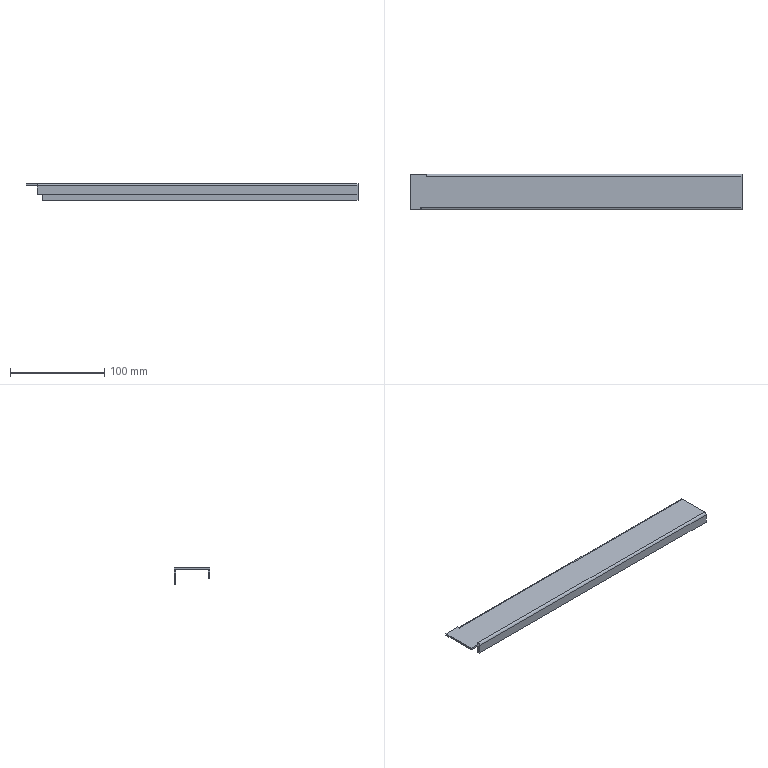Part | STEP file | Electrical Cabinet 5 | 1 solid | 22 faces | box 352 x 38 x 18 mm | volume 43368 mm3 | plane 18 | cylinder 4 | commonest cylinder face diameters 1 x2 5 x2
STEP:
#1=CARTESIAN_POINT('',(-50.375,-23.063,-2.));
#2=VERTEX_POINT('',#1);
#3=CARTESIAN_POINT('',(-38.775,-23.063,-2.));
#4=VERTEX_POINT('',#3);
#5=CARTESIAN_POINT('',(0.,-23.063,-2.));
#6=DIRECTION('',(1.,0.,0.));
#7=VECTOR('',#6,1000.);
#8=LINE('',#5,#7);
#9=EDGE_CURVE('',#2,#4,#8,.T.);
#10=ORIENTED_EDGE('',*,*,#9,.F.);
#11=CARTESIAN_POINT('',(-50.375,14.937,-2.));
#12=VERTEX_POINT('',#11);
#13=CARTESIAN_POINT('',(-50.375,0.,-2.));
#14=DIRECTION('',(0.,-1.,0.));
#15=VECTOR('',#14,1000.);
#16=LINE('',#13,#15);
#17=EDGE_CURVE('',#12,#2,#16,.T.);
#18=ORIENTED_EDGE('',*,*,#17,.F.);
#19=CARTESIAN_POINT('',(-32.775,14.937,-2.));
#20=VERTEX_POINT('',#19);
#21=CARTESIAN_POINT('',(0.,14.937,-2.));
#22=DIRECTION('',(-1.,0.,0.));
#23=VECTOR('',#22,1000.);
#24=LINE('',#21,#23);
#25=EDGE_CURVE('',#20,#12,#24,.T.);
#26=ORIENTED_EDGE('',*,*,#25,.F.);
#27=CARTESIAN_POINT('',(-32.775,12.037,-2.));
#28=VERTEX_POINT('',#27);
#29=CARTESIAN_POINT('',(-32.775,0.,-2.));
#30=DIRECTION('',(0.,1.,0.));
#31=VECTOR('',#30,1000.);
#32=LINE('',#29,#31);
#33=EDGE_CURVE('',#28,#20,#32,.T.);
#34=ORIENTED_EDGE('',*,*,#33,.F.);
#35=CARTESIAN_POINT('',(-32.375,12.037,-2.));
#36=VERTEX_POINT('',#35);
#37=CARTESIAN_POINT('',(-32.375,12.037,-2.));
#38=DIRECTION('',(-1.,0.,0.));
#39=VECTOR('',#38,1000.);
#40=LINE('',#37,#39);
#41=EDGE_CURVE('',#36,#28,#40,.T.);
#42=ORIENTED_EDGE('',*,*,#41,.F.);
#43=CARTESIAN_POINT('',(-32.375,12.437,-2.));
#44=VERTEX_POINT('',#43);
#45=CARTESIAN_POINT('',(-32.375,12.437,-2.));
#46=DIRECTION('',(0.,-1.,0.));
#47=VECTOR('',#46,1000.);
#48=LINE('',#45,#47);
#49=EDGE_CURVE('',#44,#36,#48,.T.);
#50=ORIENTED_EDGE('',*,*,#49,.F.);
#51=CARTESIAN_POINT('',(301.625,12.437,-2.));
#52=VERTEX_POINT('',#51);
#53=CARTESIAN_POINT('',(0.,12.437,-2.));
#54=DIRECTION('',(-1.,0.,0.));
#55=VECTOR('',#54,1000.);
#56=LINE('',#53,#55);
#57=EDGE_CURVE('',#52,#44,#56,.T.);
#58=ORIENTED_EDGE('',*,*,#57,.F.);
#59=CARTESIAN_POINT('',(301.625,-20.563,-2.));
#60=VERTEX_POINT('',#59);
#61=CARTESIAN_POINT('',(301.625,0.,-2.));
#62=DIRECTION('',(0.,1.,0.));
#63=VECTOR('',#62,1000.);
#64=LINE('',#61,#63);
#65=EDGE_CURVE('',#60,#52,#64,.T.);
#66=ORIENTED_EDGE('',*,*,#65,.F.);
#67=CARTESIAN_POINT('',(-38.375,-20.563,-2.));
#68=VERTEX_POINT('',#67);
#69=CARTESIAN_POINT('',(0.,-20.563,-2.));
#70=DIRECTION('',(1.,0.,0.));
#71=VECTOR('',#70,1000.);
#72=LINE('',#69,#71);
#73=EDGE_CURVE('',#68,#60,#72,.T.);
#74=ORIENTED_EDGE('',*,*,#73,.F.);
#75=CARTESIAN_POINT('',(-38.375,-20.163,-2.));
#76=VERTEX_POINT('',#75);
#77=CARTESIAN_POINT('',(-38.375,-20.163,-2.));
#78=DIRECTION('',(0.,-1.,0.));
#79=VECTOR('',#78,1000.);
#80=LINE('',#77,#79);
#81=EDGE_CURVE('',#76,#68,#80,.T.);
#82=ORIENTED_EDGE('',*,*,#81,.F.);
#83=CARTESIAN_POINT('',(-38.775,-20.163,-2.));
#84=VERTEX_POINT('',#83);
#85=CARTESIAN_POINT('',(-38.775,-20.163,-2.));
#86=DIRECTION('',(1.,0.,0.));
#87=VECTOR('',#86,1000.);
#88=LINE('',#85,#87);
#89=EDGE_CURVE('',#84,#76,#88,.T.);
#90=ORIENTED_EDGE('',*,*,#89,.F.);
#91=CARTESIAN_POINT('',(-38.775,0.,-2.));
#92=DIRECTION('',(0.,1.,0.));
#93=VECTOR('',#92,1000.);
#94=LINE('',#91,#93);
#95=EDGE_CURVE('',#4,#84,#94,.T.);
#96=ORIENTED_EDGE('',*,*,#95,.F.);
#97=EDGE_LOOP('',(#10,#18,#26,#34,#42,#50,#58,#66,#74,#82,#90,#96));
#98=FACE_OUTER_BOUND('',#97,.T.);
#99=CARTESIAN_POINT('',(0.,0.,-2.));
#100=DIRECTION('',(0.,0.,1.));
#101=DIRECTION('',(1.,0.,0.));
#102=AXIS2_PLACEMENT_3D('',#99,#100,#101);
#103=PLANE('',#102);
#104=ADVANCED_FACE('',(#98),#103,.F.);
#105=ORIENTED_EDGE('',*,*,#95,.T.);
#106=CARTESIAN_POINT('',(-38.775,-20.163,0.));
#107=VERTEX_POINT('',#106);
#108=CARTESIAN_POINT('',(-38.775,-20.163,-2.));
#109=DIRECTION('',(0.,0.,1.));
#110=VECTOR('',#109,1000.);
#111=LINE('',#108,#110);
#112=EDGE_CURVE('',#84,#107,#111,.T.);
#113=ORIENTED_EDGE('',*,*,#112,.T.);
#114=CARTESIAN_POINT('',(-38.775,-23.063,0.));
#115=VERTEX_POINT('',#114);
#116=CARTESIAN_POINT('',(-38.775,-23.063,0.));
#117=DIRECTION('',(0.,-1.,0.));
#118=VECTOR('',#117,1000.);
#119=LINE('',#116,#118);
#120=EDGE_CURVE('',#107,#115,#119,.T.);
#121=ORIENTED_EDGE('',*,*,#120,.T.);
#122=CARTESIAN_POINT('',(-38.775,-23.063,-2.));
#123=DIRECTION('',(0.,0.,-1.));
#124=VECTOR('',#123,1000.);
#125=LINE('',#122,#124);
#126=EDGE_CURVE('',#115,#4,#125,.T.);
#127=ORIENTED_EDGE('',*,*,#126,.T.);
#128=EDGE_LOOP('',(#105,#113,#121,#127));
#129=FACE_OUTER_BOUND('',#128,.T.);
#130=CARTESIAN_POINT('',(-38.775,-23.063,-2.));
#131=DIRECTION('',(1.,0.,0.));
#132=DIRECTION('',(0.,0.,-1.));
#133=AXIS2_PLACEMENT_3D('',#130,#131,#132);
#134=PLANE('',#133);
#135=ADVANCED_FACE('',(#129),#134,.T.);
#136=CARTESIAN_POINT('',(-50.375,-23.063,0.));
#137=VERTEX_POINT('',#136);
#138=CARTESIAN_POINT('',(-50.375,-23.063,0.));
#139=DIRECTION('',(-1.,0.,0.));
#140=VECTOR('',#139,1000.);
#141=LINE('',#138,#140);
#142=EDGE_CURVE('',#115,#137,#141,.T.);
#143=ORIENTED_EDGE('',*,*,#142,.T.);
#144=CARTESIAN_POINT('',(-50.375,-23.063,-2.));
#145=DIRECTION('',(0.,0.,-1.));
#146=VECTOR('',#145,1000.);
#147=LINE('',#144,#146);
#148=EDGE_CURVE('',#137,#2,#147,.T.);
#149=ORIENTED_EDGE('',*,*,#148,.T.);
#150=ORIENTED_EDGE('',*,*,#9,.T.);
#151=ORIENTED_EDGE('',*,*,#126,.F.);
#152=EDGE_LOOP('',(#143,#149,#150,#151));
#153=FACE_OUTER_BOUND('',#152,.T.);
#154=CARTESIAN_POINT('',(-50.375,-23.063,-2.));
#155=DIRECTION('',(0.,-1.,0.));
#156=DIRECTION('',(0.,0.,-1.));
#157=AXIS2_PLACEMENT_3D('',#154,#155,#156);
#158=PLANE('',#157);
#159=ADVANCED_FACE('',(#153),#158,.T.);
#160=ORIENTED_EDGE('',*,*,#17,.T.);
#161=ORIENTED_EDGE('',*,*,#148,.F.);
#162=CARTESIAN_POINT('',(-50.375,14.937,0.));
#163=VERTEX_POINT('',#162);
#164=CARTESIAN_POINT('',(-50.375,14.937,0.));
#165=DIRECTION('',(0.,1.,0.));
#166=VECTOR('',#165,1000.);
#167=LINE('',#164,#166);
#168=EDGE_CURVE('',#137,#163,#167,.T.);
#169=ORIENTED_EDGE('',*,*,#168,.T.);
#170=CARTESIAN_POINT('',(-50.375,14.937,-2.));
#171=DIRECTION('',(0.,0.,-1.));
#172=VECTOR('',#171,1000.);
#173=LINE('',#170,#172);
#174=EDGE_CURVE('',#163,#12,#173,.T.);
#175=ORIENTED_EDGE('',*,*,#174,.T.);
#176=EDGE_LOOP('',(#160,#161,#169,#175));
#177=FACE_OUTER_BOUND('',#176,.T.);
#178=CARTESIAN_POINT('',(-50.375,14.937,-2.));
#179=DIRECTION('',(-1.,0.,0.));
#180=DIRECTION('',(0.,-1.,0.));
#181=AXIS2_PLACEMENT_3D('',#178,#179,#180);
#182=PLANE('',#181);
#183=ADVANCED_FACE('',(#177),#182,.T.);
#184=ORIENTED_EDGE('',*,*,#25,.T.);
#185=ORIENTED_EDGE('',*,*,#174,.F.);
#186=CARTESIAN_POINT('',(-32.775,14.937,0.));
#187=VERTEX_POINT('',#186);
#188=CARTESIAN_POINT('',(-50.375,14.937,0.));
#189=DIRECTION('',(1.,0.,0.));
#190=VECTOR('',#189,1000.);
#191=LINE('',#188,#190);
#192=EDGE_CURVE('',#163,#187,#191,.T.);
#193=ORIENTED_EDGE('',*,*,#192,.T.);
#194=CARTESIAN_POINT('',(-32.775,14.937,-2.));
#195=DIRECTION('',(0.,0.,-1.));
#196=VECTOR('',#195,1000.);
#197=LINE('',#194,#196);
#198=EDGE_CURVE('',#187,#20,#197,.T.);
#199=ORIENTED_EDGE('',*,*,#198,.T.);
#200=EDGE_LOOP('',(#184,#185,#193,#199));
#201=FACE_OUTER_BOUND('',#200,.T.);
#202=CARTESIAN_POINT('',(-50.375,14.937,-2.));
#203=DIRECTION('',(0.,1.,0.));
#204=DIRECTION('',(0.,0.,1.));
#205=AXIS2_PLACEMENT_3D('',#202,#203,#204);
#206=PLANE('',#205);
#207=ADVANCED_FACE('',(#201),#206,.T.);
#208=ORIENTED_EDGE('',*,*,#33,.T.);
#209=ORIENTED_EDGE('',*,*,#198,.F.);
#210=CARTESIAN_POINT('',(-32.775,12.037,0.));
#211=VERTEX_POINT('',#210);
#212=CARTESIAN_POINT('',(-32.775,12.037,0.));
#213=DIRECTION('',(0.,-1.,0.));
#214=VECTOR('',#213,1000.);
#215=LINE('',#212,#214);
#216=EDGE_CURVE('',#187,#211,#215,.T.);
#217=ORIENTED_EDGE('',*,*,#216,.T.);
#218=CARTESIAN_POINT('',(-32.775,12.037,-2.));
#219=DIRECTION('',(0.,0.,-1.));
#220=VECTOR('',#219,1000.);
#221=LINE('',#218,#220);
#222=EDGE_CURVE('',#211,#28,#221,.T.);
#223=ORIENTED_EDGE('',*,*,#222,.T.);
#224=EDGE_LOOP('',(#208,#209,#217,#223));
#225=FACE_OUTER_BOUND('',#224,.T.);
#226=CARTESIAN_POINT('',(-32.775,12.037,-2.));
#227=DIRECTION('',(1.,0.,0.));
#228=DIRECTION('',(0.,0.,-1.));
#229=AXIS2_PLACEMENT_3D('',#226,#227,#228);
#230=PLANE('',#229);
#231=ADVANCED_FACE('',(#225),#230,.T.);
#232=CARTESIAN_POINT('',(-32.375,12.937,-2.5));
#233=VERTEX_POINT('',#232);
#234=CARTESIAN_POINT('',(-32.375,12.437,-2.5));
#235=DIRECTION('',(1.,0.,0.));
#236=DIRECTION('',(0.,0.,-1.));
#237=AXIS2_PLACEMENT_3D('',#234,#235,#236);
#238=CIRCLE('',#237,0.5);
#239=EDGE_CURVE('',#233,#44,#238,.T.);
#240=ORIENTED_EDGE('',*,*,#239,.F.);
#241=CARTESIAN_POINT('',(301.625,12.937,-2.5));
#242=VERTEX_POINT('',#241);
#243=CARTESIAN_POINT('',(301.625,12.937,-2.5));
#244=DIRECTION('',(-1.,0.,0.));
#245=VECTOR('',#244,1000.);
#246=LINE('',#243,#245);
#247=EDGE_CURVE('',#242,#233,#246,.T.);
#248=ORIENTED_EDGE('',*,*,#247,.F.);
#249=CARTESIAN_POINT('',(301.625,12.437,-2.5));
#250=DIRECTION('',(1.,0.,0.));
#251=DIRECTION('',(0.,0.,-1.));
#252=AXIS2_PLACEMENT_3D('',#249,#250,#251);
#253=CIRCLE('',#252,0.5);
#254=EDGE_CURVE('',#242,#52,#253,.T.);
#255=ORIENTED_EDGE('',*,*,#254,.T.);
#256=ORIENTED_EDGE('',*,*,#57,.T.);
#257=EDGE_LOOP('',(#240,#248,#255,#256));
#258=FACE_OUTER_BOUND('',#257,.T.);
#259=CARTESIAN_POINT('',(301.625,12.437,-2.5));
#260=DIRECTION('',(1.,0.,0.));
#261=DIRECTION('',(0.,0.,-1.));
#262=AXIS2_PLACEMENT_3D('',#259,#260,#261);
#263=CYLINDRICAL_SURFACE('',#262,0.5);
#264=ADVANCED_FACE('',(#258),#263,.F.);
#265=ORIENTED_EDGE('',*,*,#65,.T.);
#266=ORIENTED_EDGE('',*,*,#254,.F.);
#267=CARTESIAN_POINT('',(301.625,12.937,-18.));
#268=VERTEX_POINT('',#267);
#269=CARTESIAN_POINT('',(301.625,12.937,0.));
#270=DIRECTION('',(0.,0.,-1.));
#271=VECTOR('',#270,1000.);
#272=LINE('',#269,#271);
#273=EDGE_CURVE('',#242,#268,#272,.T.);
#274=ORIENTED_EDGE('',*,*,#273,.T.);
#275=CARTESIAN_POINT('',(301.625,14.937,-18.));
#276=VERTEX_POINT('',#275);
#277=CARTESIAN_POINT('',(301.625,14.937,-18.));
#278=DIRECTION('',(0.,-1.,0.));
#279=VECTOR('',#278,1000.);
#280=LINE('',#277,#279);
#281=EDGE_CURVE('',#276,#268,#280,.T.);
#282=ORIENTED_EDGE('',*,*,#281,.F.);
#283=CARTESIAN_POINT('',(301.625,14.937,-2.5));
#284=VERTEX_POINT('',#283);
#285=CARTESIAN_POINT('',(301.625,14.937,-2.));
#286=DIRECTION('',(0.,0.,1.));
#287=VECTOR('',#286,1000.);
#288=LINE('',#285,#287);
#289=EDGE_CURVE('',#276,#284,#288,.T.);
#290=ORIENTED_EDGE('',*,*,#289,.T.);
#291=CARTESIAN_POINT('',(301.625,12.437,0.));
#292=VERTEX_POINT('',#291);
#293=CARTESIAN_POINT('',(301.625,12.437,-2.5));
#294=DIRECTION('',(-1.,0.,0.));
#295=DIRECTION('',(0.,0.,-1.));
#296=AXIS2_PLACEMENT_3D('',#293,#294,#295);
#297=CIRCLE('',#296,2.5);
#298=EDGE_CURVE('',#292,#284,#297,.T.);
#299=ORIENTED_EDGE('',*,*,#298,.F.);
#300=CARTESIAN_POINT('',(301.625,-20.563,0.));
#301=VERTEX_POINT('',#300);
#302=CARTESIAN_POINT('',(301.625,14.937,0.));
#303=DIRECTION('',(0.,-1.,0.));
#304=VECTOR('',#303,1000.);
#305=LINE('',#302,#304);
#306=EDGE_CURVE('',#292,#301,#305,.T.);
#307=ORIENTED_EDGE('',*,*,#306,.T.);
#308=CARTESIAN_POINT('',(301.625,-23.063,-2.5));
#309=VERTEX_POINT('',#308);
#310=CARTESIAN_POINT('',(301.625,-20.563,-2.5));
#311=DIRECTION('',(1.,0.,0.));
#312=DIRECTION('',(0.,0.,1.));
#313=AXIS2_PLACEMENT_3D('',#310,#311,#312);
#314=CIRCLE('',#313,2.5);
#315=EDGE_CURVE('',#301,#309,#314,.T.);
#316=ORIENTED_EDGE('',*,*,#315,.T.);
#317=CARTESIAN_POINT('',(301.625,-23.063,-12.));
#318=VERTEX_POINT('',#317);
#319=CARTESIAN_POINT('',(301.625,-23.063,-2.));
#320=DIRECTION('',(0.,0.,1.));
#321=VECTOR('',#320,1000.);
#322=LINE('',#319,#321);
#323=EDGE_CURVE('',#318,#309,#322,.T.);
#324=ORIENTED_EDGE('',*,*,#323,.F.);
#325=CARTESIAN_POINT('',(301.625,-21.063,-12.));
#326=VERTEX_POINT('',#325);
#327=CARTESIAN_POINT('',(301.625,-23.063,-12.));
#328=DIRECTION('',(0.,-1.,0.));
#329=VECTOR('',#328,1000.);
#330=LINE('',#327,#329);
#331=EDGE_CURVE('',#326,#318,#330,.T.);
#332=ORIENTED_EDGE('',*,*,#331,.F.);
#333=CARTESIAN_POINT('',(301.625,-21.063,-2.5));
#334=VERTEX_POINT('',#333);
#335=CARTESIAN_POINT('',(301.625,-21.063,0.));
#336=DIRECTION('',(0.,0.,-1.));
#337=VECTOR('',#336,1000.);
#338=LINE('',#335,#337);
#339=EDGE_CURVE('',#334,#326,#338,.T.);
#340=ORIENTED_EDGE('',*,*,#339,.F.);
#341=CARTESIAN_POINT('',(301.625,-20.563,-2.5));
#342=DIRECTION('',(-1.,0.,0.));
#343=DIRECTION('',(0.,0.,1.));
#344=AXIS2_PLACEMENT_3D('',#341,#342,#343);
#345=CIRCLE('',#344,0.5);
#346=EDGE_CURVE('',#334,#60,#345,.T.);
#347=ORIENTED_EDGE('',*,*,#346,.T.);
#348=EDGE_LOOP('',(#265,#266,#274,#282,#290,#299,#307,#316,#324,#332,#340,#347));
#349=FACE_OUTER_BOUND('',#348,.T.);
#350=CARTESIAN_POINT('',(301.625,14.937,-2.));
#351=DIRECTION('',(1.,0.,0.));
#352=DIRECTION('',(0.,0.,-1.));
#353=AXIS2_PLACEMENT_3D('',#350,#351,#352);
#354=PLANE('',#353);
#355=ADVANCED_FACE('',(#349),#354,.T.);
#356=ORIENTED_EDGE('',*,*,#346,.F.);
#357=CARTESIAN_POINT('',(-38.375,-21.063,-2.5));
#358=VERTEX_POINT('',#357);
#359=CARTESIAN_POINT('',(-38.375,-21.063,-2.5));
#360=DIRECTION('',(1.,0.,0.));
#361=VECTOR('',#360,1000.);
#362=LINE('',#359,#361);
#363=EDGE_CURVE('',#358,#334,#362,.T.);
#364=ORIENTED_EDGE('',*,*,#363,.F.);
#365=CARTESIAN_POINT('',(-38.375,-20.563,-2.5));
#366=DIRECTION('',(-1.,0.,0.));
#367=DIRECTION('',(0.,0.,1.));
#368=AXIS2_PLACEMENT_3D('',#365,#366,#367);
#369=CIRCLE('',#368,0.5);
#370=EDGE_CURVE('',#358,#68,#369,.T.);
#371=ORIENTED_EDGE('',*,*,#370,.T.);
#372=ORIENTED_EDGE('',*,*,#73,.T.);
#373=EDGE_LOOP('',(#356,#364,#371,#372));
#374=FACE_OUTER_BOUND('',#373,.T.);
#375=CARTESIAN_POINT('',(-38.375,-20.563,-2.5));
#376=DIRECTION('',(-1.,0.,0.));
#377=DIRECTION('',(0.,0.,1.));
#378=AXIS2_PLACEMENT_3D('',#375,#376,#377);
#379=CYLINDRICAL_SURFACE('',#378,0.5);
#380=ADVANCED_FACE('',(#374),#379,.F.);
#381=ORIENTED_EDGE('',*,*,#89,.T.);
#382=CARTESIAN_POINT('',(-38.375,-20.163,0.));
#383=VERTEX_POINT('',#382);
#384=CARTESIAN_POINT('',(-38.375,-20.163,-2.));
#385=DIRECTION('',(0.,0.,1.));
#386=VECTOR('',#385,1000.);
#387=LINE('',#384,#386);
#388=EDGE_CURVE('',#76,#383,#387,.T.);
#389=ORIENTED_EDGE('',*,*,#388,.T.);
#390=CARTESIAN_POINT('',(-38.775,-20.163,0.));
#391=DIRECTION('',(-1.,0.,0.));
#392=VECTOR('',#391,1000.);
#393=LINE('',#390,#392);
#394=EDGE_CURVE('',#383,#107,#393,.T.);
#395=ORIENTED_EDGE('',*,*,#394,.T.);
#396=ORIENTED_EDGE('',*,*,#112,.F.);
#397=EDGE_LOOP('',(#381,#389,#395,#396));
#398=FACE_OUTER_BOUND('',#397,.T.);
#399=CARTESIAN_POINT('',(-38.775,-20.163,-2.));
#400=DIRECTION('',(0.,-1.,0.));
#401=DIRECTION('',(0.,0.,-1.));
#402=AXIS2_PLACEMENT_3D('',#399,#400,#401);
#403=PLANE('',#402);
#404=ADVANCED_FACE('',(#398),#403,.T.);
#405=ORIENTED_EDGE('',*,*,#192,.F.);
#406=ORIENTED_EDGE('',*,*,#168,.F.);
#407=ORIENTED_EDGE('',*,*,#142,.F.);
#408=ORIENTED_EDGE('',*,*,#120,.F.);
#409=ORIENTED_EDGE('',*,*,#394,.F.);
#410=CARTESIAN_POINT('',(-38.375,-20.563,0.));
#411=VERTEX_POINT('',#410);
#412=CARTESIAN_POINT('',(-38.375,0.,0.));
#413=DIRECTION('',(0.,-1.,0.));
#414=VECTOR('',#413,1000.);
#415=LINE('',#412,#414);
#416=EDGE_CURVE('',#383,#411,#415,.T.);
#417=ORIENTED_EDGE('',*,*,#416,.T.);
#418=CARTESIAN_POINT('',(0.,-20.563,0.));
#419=DIRECTION('',(1.,0.,0.));
#420=VECTOR('',#419,1000.);
#421=LINE('',#418,#420);
#422=EDGE_CURVE('',#411,#301,#421,.T.);
#423=ORIENTED_EDGE('',*,*,#422,.T.);
#424=ORIENTED_EDGE('',*,*,#306,.F.);
#425=CARTESIAN_POINT('',(-32.375,12.437,0.));
#426=VERTEX_POINT('',#425);
#427=CARTESIAN_POINT('',(0.,12.437,0.));
#428=DIRECTION('',(-1.,0.,0.));
#429=VECTOR('',#428,1000.);
#430=LINE('',#427,#429);
#431=EDGE_CURVE('',#292,#426,#430,.T.);
#432=ORIENTED_EDGE('',*,*,#431,.T.);
#433=CARTESIAN_POINT('',(-32.375,12.037,0.));
#434=VERTEX_POINT('',#433);
#435=CARTESIAN_POINT('',(-32.375,12.437,0.));
#436=DIRECTION('',(0.,1.,0.));
#437=VECTOR('',#436,1000.);
#438=LINE('',#435,#437);
#439=EDGE_CURVE('',#434,#426,#438,.T.);
#440=ORIENTED_EDGE('',*,*,#439,.F.);
#441=CARTESIAN_POINT('',(0.,12.037,0.));
#442=DIRECTION('',(-1.,0.,0.));
#443=VECTOR('',#442,1000.);
#444=LINE('',#441,#443);
#445=EDGE_CURVE('',#434,#211,#444,.T.);
#446=ORIENTED_EDGE('',*,*,#445,.T.);
#447=ORIENTED_EDGE('',*,*,#216,.F.);
#448=EDGE_LOOP('',(#405,#406,#407,#408,#409,#417,#423,#424,#432,#440,#446,#447));
#449=FACE_OUTER_BOUND('',#448,.T.);
#450=CARTESIAN_POINT('',(0.,0.,0.));
#451=DIRECTION('',(0.,0.,1.));
#452=DIRECTION('',(1.,0.,0.));
#453=AXIS2_PLACEMENT_3D('',#450,#451,#452);
#454=PLANE('',#453);
#455=ADVANCED_FACE('',(#449),#454,.T.);
#456=ORIENTED_EDGE('',*,*,#41,.T.);
#457=ORIENTED_EDGE('',*,*,#222,.F.);
#458=ORIENTED_EDGE('',*,*,#445,.F.);
#459=CARTESIAN_POINT('',(-32.375,12.037,-2.));
#460=DIRECTION('',(0.,0.,-1.));
#461=VECTOR('',#460,1000.);
#462=LINE('',#459,#461);
#463=EDGE_CURVE('',#434,#36,#462,.T.);
#464=ORIENTED_EDGE('',*,*,#463,.T.);
#465=EDGE_LOOP('',(#456,#457,#458,#464));
#466=FACE_OUTER_BOUND('',#465,.T.);
#467=CARTESIAN_POINT('',(-32.375,12.037,-2.));
#468=DIRECTION('',(0.,1.,0.));
#469=DIRECTION('',(0.,0.,1.));
#470=AXIS2_PLACEMENT_3D('',#467,#468,#469);
#471=PLANE('',#470);
#472=ADVANCED_FACE('',(#466),#471,.T.);
#473=CARTESIAN_POINT('',(-32.375,12.937,-18.));
#474=VERTEX_POINT('',#473);
#475=CARTESIAN_POINT('',(-32.375,12.937,0.));
#476=DIRECTION('',(0.,0.,1.));
#477=VECTOR('',#476,1000.);
#478=LINE('',#475,#477);
#479=EDGE_CURVE('',#474,#233,#478,.T.);
#480=ORIENTED_EDGE('',*,*,#479,.F.);
#481=CARTESIAN_POINT('',(0.,12.937,-18.));
#482=DIRECTION('',(-1.,0.,0.));
#483=VECTOR('',#482,1000.);
#484=LINE('',#481,#483);
#485=EDGE_CURVE('',#268,#474,#484,.T.);
#486=ORIENTED_EDGE('',*,*,#485,.F.);
#487=ORIENTED_EDGE('',*,*,#273,.F.);
#488=ORIENTED_EDGE('',*,*,#247,.T.);
#489=EDGE_LOOP('',(#480,#486,#487,#488));
#490=FACE_OUTER_BOUND('',#489,.T.);
#491=CARTESIAN_POINT('',(0.,12.937,0.));
#492=DIRECTION('',(0.,1.,0.));
#493=DIRECTION('',(0.,0.,1.));
#494=AXIS2_PLACEMENT_3D('',#491,#492,#493);
#495=PLANE('',#494);
#496=ADVANCED_FACE('',(#490),#495,.F.);
#497=ORIENTED_EDGE('',*,*,#339,.T.);
#498=CARTESIAN_POINT('',(-38.375,-21.063,-12.));
#499=VERTEX_POINT('',#498);
#500=CARTESIAN_POINT('',(0.,-21.063,-12.));
#501=DIRECTION('',(-1.,0.,0.));
#502=VECTOR('',#501,1000.);
#503=LINE('',#500,#502);
#504=EDGE_CURVE('',#326,#499,#503,.T.);
#505=ORIENTED_EDGE('',*,*,#504,.T.);
#506=CARTESIAN_POINT('',(-38.375,-21.063,0.));
#507=DIRECTION('',(0.,0.,1.));
#508=VECTOR('',#507,1000.);
#509=LINE('',#506,#508);
#510=EDGE_CURVE('',#499,#358,#509,.T.);
#511=ORIENTED_EDGE('',*,*,#510,.T.);
#512=ORIENTED_EDGE('',*,*,#363,.T.);
#513=EDGE_LOOP('',(#497,#505,#511,#512));
#514=FACE_OUTER_BOUND('',#513,.T.);
#515=CARTESIAN_POINT('',(0.,-21.063,0.));
#516=DIRECTION('',(0.,1.,0.));
#517=DIRECTION('',(0.,0.,1.));
#518=AXIS2_PLACEMENT_3D('',#515,#516,#517);
#519=PLANE('',#518);
#520=ADVANCED_FACE('',(#514),#519,.T.);
#521=ORIENTED_EDGE('',*,*,#81,.T.);
#522=ORIENTED_EDGE('',*,*,#370,.F.);
#523=ORIENTED_EDGE('',*,*,#510,.F.);
#524=CARTESIAN_POINT('',(-38.375,-23.063,-12.));
#525=VERTEX_POINT('',#524);
#526=CARTESIAN_POINT('',(-38.375,-23.063,-12.));
#527=DIRECTION('',(0.,-1.,0.));
#528=VECTOR('',#527,1000.);
#529=LINE('',#526,#528);
#530=EDGE_CURVE('',#499,#525,#529,.T.);
#531=ORIENTED_EDGE('',*,*,#530,.T.);
#532=CARTESIAN_POINT('',(-38.375,-23.063,-2.5));
#533=VERTEX_POINT('',#532);
#534=CARTESIAN_POINT('',(-38.375,-23.063,-12.));
#535=DIRECTION('',(0.,0.,-1.));
#536=VECTOR('',#535,1000.);
#537=LINE('',#534,#536);
#538=EDGE_CURVE('',#533,#525,#537,.T.);
#539=ORIENTED_EDGE('',*,*,#538,.F.);
#540=CARTESIAN_POINT('',(-38.375,-20.563,-2.5));
#541=DIRECTION('',(1.,0.,0.));
#542=DIRECTION('',(0.,0.,1.));
#543=AXIS2_PLACEMENT_3D('',#540,#541,#542);
#544=CIRCLE('',#543,2.5);
#545=EDGE_CURVE('',#411,#533,#544,.T.);
#546=ORIENTED_EDGE('',*,*,#545,.F.);
#547=ORIENTED_EDGE('',*,*,#416,.F.);
#548=ORIENTED_EDGE('',*,*,#388,.F.);
#549=EDGE_LOOP('',(#521,#522,#523,#531,#539,#546,#547,#548));
#550=FACE_OUTER_BOUND('',#549,.T.);
#551=CARTESIAN_POINT('',(-38.375,-20.163,-2.));
#552=DIRECTION('',(-1.,0.,0.));
#553=DIRECTION('',(0.,0.,1.));
#554=AXIS2_PLACEMENT_3D('',#551,#552,#553);
#555=PLANE('',#554);
#556=ADVANCED_FACE('',(#550),#555,.T.);
#557=CARTESIAN_POINT('',(-32.375,14.937,-2.5));
#558=VERTEX_POINT('',#557);
#559=CARTESIAN_POINT('',(301.625,14.937,-2.5));
#560=DIRECTION('',(-1.,0.,0.));
#561=VECTOR('',#560,1000.);
#562=LINE('',#559,#561);
#563=EDGE_CURVE('',#284,#558,#562,.T.);
#564=ORIENTED_EDGE('',*,*,#563,.T.);
#565=CARTESIAN_POINT('',(-32.375,12.437,-2.5));
#566=DIRECTION('',(1.,0.,0.));
#567=DIRECTION('',(0.,0.,-1.));
#568=AXIS2_PLACEMENT_3D('',#565,#566,#567);
#569=CIRCLE('',#568,2.5);
#570=EDGE_CURVE('',#558,#426,#569,.T.);
#571=ORIENTED_EDGE('',*,*,#570,.T.);
#572=ORIENTED_EDGE('',*,*,#431,.F.);
#573=ORIENTED_EDGE('',*,*,#298,.T.);
#574=EDGE_LOOP('',(#564,#571,#572,#573));
#575=FACE_OUTER_BOUND('',#574,.T.);
#576=CARTESIAN_POINT('',(301.625,12.437,-2.5));
#577=DIRECTION('',(1.,0.,0.));
#578=DIRECTION('',(0.,0.,-1.));
#579=AXIS2_PLACEMENT_3D('',#576,#577,#578);
#580=CYLINDRICAL_SURFACE('',#579,2.5);
#581=ADVANCED_FACE('',(#575),#580,.T.);
#582=CARTESIAN_POINT('',(-38.375,-23.063,-2.5));
#583=DIRECTION('',(1.,0.,0.));
#584=VECTOR('',#583,1000.);
#585=LINE('',#582,#584);
#586=EDGE_CURVE('',#533,#309,#585,.T.);
#587=ORIENTED_EDGE('',*,*,#586,.T.);
#588=ORIENTED_EDGE('',*,*,#315,.F.);
#589=ORIENTED_EDGE('',*,*,#422,.F.);
#590=ORIENTED_EDGE('',*,*,#545,.T.);
#591=EDGE_LOOP('',(#587,#588,#589,#590));
#592=FACE_OUTER_BOUND('',#591,.T.);
#593=CARTESIAN_POINT('',(-38.375,-20.563,-2.5));
#594=DIRECTION('',(-1.,0.,0.));
#595=DIRECTION('',(0.,0.,1.));
#596=AXIS2_PLACEMENT_3D('',#593,#594,#595);
#597=CYLINDRICAL_SURFACE('',#596,2.5);
#598=ADVANCED_FACE('',(#592),#597,.T.);
#599=ORIENTED_EDGE('',*,*,#49,.T.);
#600=ORIENTED_EDGE('',*,*,#463,.F.);
#601=ORIENTED_EDGE('',*,*,#439,.T.);
#602=ORIENTED_EDGE('',*,*,#570,.F.);
#603=CARTESIAN_POINT('',(-32.375,14.937,-18.));
#604=VERTEX_POINT('',#603);
#605=CARTESIAN_POINT('',(-32.375,14.937,-18.));
#606=DIRECTION('',(0.,0.,-1.));
#607=VECTOR('',#606,1000.);
#608=LINE('',#605,#607);
#609=EDGE_CURVE('',#558,#604,#608,.T.);
#610=ORIENTED_EDGE('',*,*,#609,.T.);
#611=CARTESIAN_POINT('',(-32.375,14.937,-18.));
#612=DIRECTION('',(0.,-1.,0.));
#613=VECTOR('',#612,1000.);
#614=LINE('',#611,#613);
#615=EDGE_CURVE('',#604,#474,#614,.T.);
#616=ORIENTED_EDGE('',*,*,#615,.T.);
#617=ORIENTED_EDGE('',*,*,#479,.T.);
#618=ORIENTED_EDGE('',*,*,#239,.T.);
#619=EDGE_LOOP('',(#599,#600,#601,#602,#610,#616,#617,#618));
#620=FACE_OUTER_BOUND('',#619,.T.);
#621=CARTESIAN_POINT('',(-32.375,12.437,-2.));
#622=DIRECTION('',(-1.,0.,0.));
#623=DIRECTION('',(0.,0.,1.));
#624=AXIS2_PLACEMENT_3D('',#621,#622,#623);
#625=PLANE('',#624);
#626=ADVANCED_FACE('',(#620),#625,.T.);
#627=CARTESIAN_POINT('',(301.625,14.937,-18.));
#628=DIRECTION('',(1.,0.,0.));
#629=VECTOR('',#628,1000.);
#630=LINE('',#627,#629);
#631=EDGE_CURVE('',#604,#276,#630,.T.);
#632=ORIENTED_EDGE('',*,*,#631,.T.);
#633=ORIENTED_EDGE('',*,*,#281,.T.);
#634=ORIENTED_EDGE('',*,*,#485,.T.);
#635=ORIENTED_EDGE('',*,*,#615,.F.);
#636=EDGE_LOOP('',(#632,#633,#634,#635));
#637=FACE_OUTER_BOUND('',#636,.T.);
#638=CARTESIAN_POINT('',(301.625,14.937,-18.));
#639=DIRECTION('',(0.,0.,-1.));
#640=DIRECTION('',(0.,1.,0.));
#641=AXIS2_PLACEMENT_3D('',#638,#639,#640);
#642=PLANE('',#641);
#643=ADVANCED_FACE('',(#637),#642,.T.);
#644=ORIENTED_EDGE('',*,*,#331,.T.);
#645=CARTESIAN_POINT('',(301.625,-23.063,-12.));
#646=DIRECTION('',(1.,0.,0.));
#647=VECTOR('',#646,1000.);
#648=LINE('',#645,#647);
#649=EDGE_CURVE('',#525,#318,#648,.T.);
#650=ORIENTED_EDGE('',*,*,#649,.F.);
#651=ORIENTED_EDGE('',*,*,#530,.F.);
#652=ORIENTED_EDGE('',*,*,#504,.F.);
#653=EDGE_LOOP('',(#644,#650,#651,#652));
#654=FACE_OUTER_BOUND('',#653,.T.);
#655=CARTESIAN_POINT('',(301.625,-23.063,-12.));
#656=DIRECTION('',(0.,0.,1.));
#657=DIRECTION('',(0.,-1.,0.));
#658=AXIS2_PLACEMENT_3D('',#655,#656,#657);
#659=PLANE('',#658);
#660=ADVANCED_FACE('',(#654),#659,.F.);
#661=ORIENTED_EDGE('',*,*,#289,.F.);
#662=ORIENTED_EDGE('',*,*,#631,.F.);
#663=ORIENTED_EDGE('',*,*,#609,.F.);
#664=ORIENTED_EDGE('',*,*,#563,.F.);
#665=EDGE_LOOP('',(#661,#662,#663,#664));
#666=FACE_OUTER_BOUND('',#665,.T.);
#667=CARTESIAN_POINT('',(0.,14.937,0.));
#668=DIRECTION('',(0.,1.,0.));
#669=DIRECTION('',(0.,0.,1.));
#670=AXIS2_PLACEMENT_3D('',#667,#668,#669);
#671=PLANE('',#670);
#672=ADVANCED_FACE('',(#666),#671,.T.);
#673=ORIENTED_EDGE('',*,*,#538,.T.);
#674=ORIENTED_EDGE('',*,*,#649,.T.);
#675=ORIENTED_EDGE('',*,*,#323,.T.);
#676=ORIENTED_EDGE('',*,*,#586,.F.);
#677=EDGE_LOOP('',(#673,#674,#675,#676));
#678=FACE_OUTER_BOUND('',#677,.T.);
#679=CARTESIAN_POINT('',(0.,-23.063,0.));
#680=DIRECTION('',(0.,1.,0.));
#681=DIRECTION('',(0.,0.,1.));
#682=AXIS2_PLACEMENT_3D('',#679,#680,#681);
#683=PLANE('',#682);
#684=ADVANCED_FACE('',(#678),#683,.F.);
#685=CLOSED_SHELL('',(#104,#135,#159,#183,#207,#231,#264,#355,#380,#404,#455,#472,#496,#520,#556,#581,#598,#626,#643,#660,#672,#684));
#686=MANIFOLD_SOLID_BREP('',#685);
#687=CARTESIAN_POINT('',(0.,0.,0.));
#688=DIRECTION('',(0.,0.,1.));
#689=DIRECTION('',(1.,0.,0.));
#690=AXIS2_PLACEMENT_3D('',#687,#688,#689);
#691=(LENGTH_UNIT()NAMED_UNIT(*)SI_UNIT(.MILLI.,.METRE.));
#692=UNCERTAINTY_MEASURE_WITH_UNIT(LENGTH_MEASURE(0.00001),#691,'','');
#693=(NAMED_UNIT(*)PLANE_ANGLE_UNIT()SI_UNIT($,.RADIAN.));
#694=(NAMED_UNIT(*)SI_UNIT($,.STERADIAN.)SOLID_ANGLE_UNIT());
#695=(GEOMETRIC_REPRESENTATION_CONTEXT(3)GLOBAL_UNCERTAINTY_ASSIGNED_CONTEXT((#692))GLOBAL_UNIT_ASSIGNED_CONTEXT((#691,#693,#694))REPRESENTATION_CONTEXT('',''));
#696=ADVANCED_BREP_SHAPE_REPRESENTATION('',(#686,#690),#695);